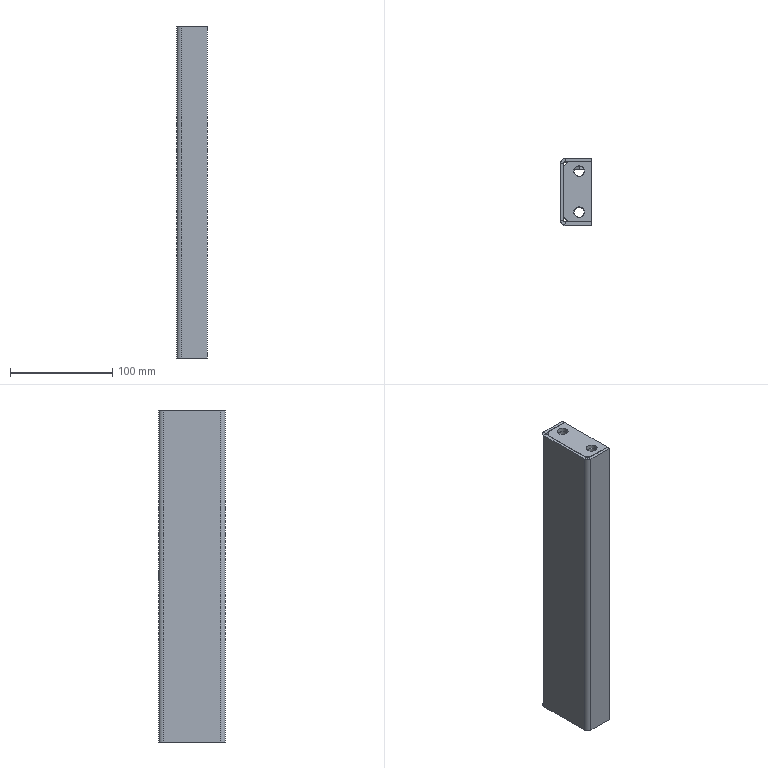Part | SolidWorks | features MoveCopyBody 5, Stock 5, FlatPattern 2, SMBaseFlange 2, SheetMetal 2, ICE 1, MirrorSolid 1 | 8 solids | 168 faces | box 30 x 65 x 324 mm | volume 129406 mm3 | plane 74 | cone 70 | cylinder 24 | commonest cylinder face diameters 10 x8 10.5 x8 9 x4 3 x2 8 x2